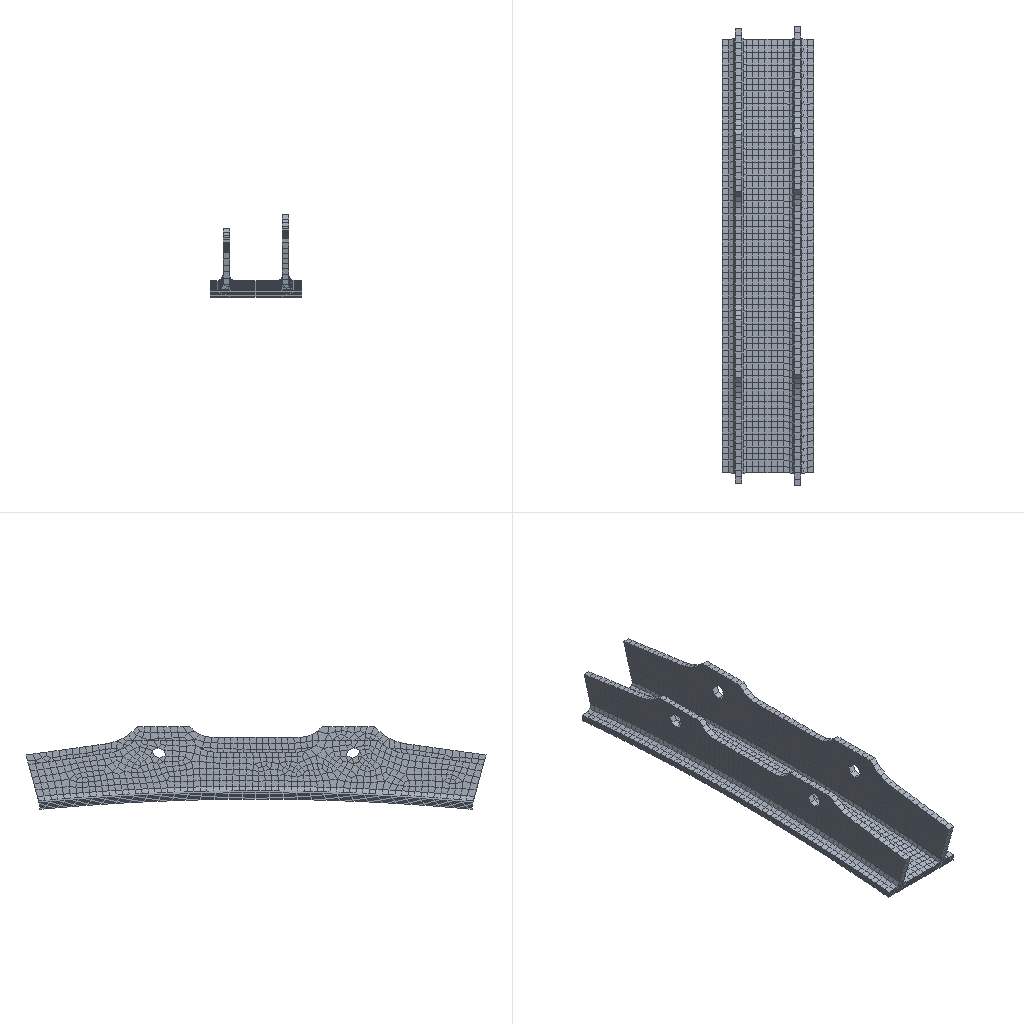Simulation study | abaqus
Set-up summary:
category,name,step,type,value,unit,region
solver,abaqus,,Abaqus/CAE 2024
units,mm-N-s-tonne (MPa),,inferred,E=250000 density=3.2e-09
analysis,Step-1,,coupled temp-displacement,time_period=24
mesh,nodes,,,11334
mesh,elements,,,8250
element_type,C3D8T,,,7245
element_type,COH3D8,,,1005
material,biaoceng,,E,250000
material,biaoceng,,nu,0.17
material,biaoceng,,density,3.2e-09
material,biaoceng,,conductivity,2
material,biaoceng,,specific_heat,7.5e+08
material,biaoceng,,cte,5e-06
material,biaoceng,,behaviors,conductivity; expansion; specific heat
material,bujian,,E,220000
material,bujian,,nu,0.17
material,bujian,,density,1.8e-09
material,bujian,,conductivity,100
material,bujian,,specific_heat,9.6e+08
material,bujian,,cte,4e-06
material,bujian,,behaviors,conductivity; expansion; specific heat
material,cohesive,,E,160000
material,cohesive,,density,2.33e-09
material,cohesive,,conductivity,148
material,cohesive,,specific_heat,7.1e+08
material,cohesive,,cte,4.6e+06
material,cohesive,,behaviors,conductivity; damage initiation; damage evolution; elastic traction; expansion; specific heat
section,bujian,,solid section,,,Set-2
section,biaoceng,,solid section,,,Set-1
section,cohesive,,cohesive section,,,CoheElem-0All
load,Predefined,initial,initial condition temperature
bc,BC-1,Step-1,displacement,1 [dofs=temp],,_PickedSet5
bc,BC-2,Step-1,encastre,[dofs=ENCASTRE],,_PickedSet6
Abaqus input file, long lists of numbers shortened:
*Heading
** Job name: deck Model name: Model-1-Copy
** Generated by: Abaqus/CAE 2024
*Preprint, echo=NO, model=NO, history=NO, contact=NO
**
** PARTS
**
*Part, name=Part1(1)-Surf(Surf-1)
*Node
      1,         -14.,   66.345,  -1.991
      2,          14.,   66.345,  -1.991
** (11332 more lines like these left out)
*Element, type=C3D8T
   1, 12174, 12118, 12182, 11854,     1,    93,  1433,   252
   2, 12118, 12120, 12184, 12182,    93,    94,  1434,  1433
** (7243 more lines like these left out)
*Element, type=COH3D8
7246, 11917, 10901, 10929, 11919, 11918, 10902, 10930, 11920
7247, 10287, 10289, 10317, 10315, 10288, 10290, 10318, 10316
** (1003 more lines like these left out)
*Elset, elset=BaseElements, generate
    1,  7245,     1
*Elset, elset=CoheElem-0All, generate
 7246,  8250,     1
*Elset, elset=Set-1, generate
 1006,  7245,     1
*Elset, elset=Set-2, generate
    1,  1005,     1
** Section: Section-3
*Solid Section, elset=Set-2, material=bujian
,
** Section: Section-1
*Solid Section, elset=Set-1, material=biaoceng
,
** Section: Section-2
*Cohesive Section, elset=CoheElem-0All, material=cohesive, response=TRACTION SEPARATION
,
*End Part
**
**
** ASSEMBLY
**
*Assembly, name=Assembly
**
*Instance, name=Part1(1)-Surf(Surf-1)-1, part=Part1(1)-Surf(Surf-1)
*End Instance
**
*Nset, nset=_PickedSet4, internal, instance=Part1(1)-Surf(Surf-1)-1
     1,     2,     3,     4,     5,     6,     7,     8,     9,    10,    11,    12,    13,    14,    15,    16
    17,    18,    19,    20,    21,    22,    23,    24,    25,    26,    27,    28,    29,    30,    31,    32
** (707 more lines like these left out)
*Nset, nset=_PickedSet5, internal, instance=Part1(1)-Surf(Surf-1)-1
    1,    2,    3,    4,   93,   94,   95,   96,   97,   98,   99,  100,  101,  102,  103,  104
  105,  106,  107,  108,  109,  110,  111,  112,  113,  114,  115,  116,  117,  118,  119,  120
** (66 more lines like these left out)
*Nset, nset=_PickedSet6, internal, instance=Part1(1)-Surf(Surf-1)-1
   33,   34,   37,   38,   46,   47,   50,   51,   65,   66,   69,   70,   77,   78,   81,   82
  774,  775,  776,  777,  778,  779,  780,  781,  800,  801,  802,  803,  804,  805,  806,  807
** (3 more lines like these left out)
*End Assembly
*Amplitude, name=Amp-1
             0.,           1000.,              8.,           1300.,             16.,           1000.,             24.,           1300.
**
** MATERIALS
**
*Material, name=biaoceng
*Conductivity
2.,
*Density
 3.2e-09,
*Elastic
250000., 0.17
*Expansion
 5e-06,
*Specific Heat
 7.5e+08,
*Material, name=bujian
*Conductivity
100.,
*Density
 1.8e-09,
*Elastic
220000., 0.17
*Expansion
 4e-06,
*Specific Heat
 9.6e+08,
*Material, name=cohesive
*Conductivity
148.,
*Damage Initiation, criterion=MAXS
50.,50.,50.
*Damage Evolution, type=DISPLACEMENT
1.,
*Density
 2.33e-09,
*Elastic, type=TRACTION
160000.,160000.,160000.
*Expansion
 4.6e+06,
*Specific Heat
 7.1e+08,
**
** PREDEFINED FIELDS
**
** Name: Predefined Field-1   Type: Temperature
*Initial Conditions, type=TEMPERATURE
_PickedSet4, 1000.
** ----------------------------------------------------------------
**
** STEP: Step-1
**
*Step, name=Step-1, nlgeom=NO, inc=10000
*Coupled Temperature-displacement, creep=none, deltmx=1000., stabilize=0.0002, allsdtol=0.05, continue=NO
0.1, 24., 0.00024, 1.
**
** BOUNDARY CONDITIONS
**
** Name: BC-1 Type: Temperature
*Boundary, amplitude=Amp-1
_PickedSet5, 11, 11, 1.
** Name: BC-2 Type: Symmetry/Antisymmetry/Encastre
*Boundary
_PickedSet6, ENCASTRE
**
** OUTPUT REQUESTS
**
*Restart, write, frequency=0
**
** FIELD OUTPUT: F-Output-1
**
*Output, field
*Node Output
CF, NT, RF, RFL, U
*Element Output, directions=YES
HFL, LE, PE, PEEQ, PEMAG, S, SDEG, STATUS
*Contact Output
CDISP, CSTRESS
**
** HISTORY OUTPUT: H-Output-1
**
*Output, history, variable=PRESELECT
*End Step
Results summary:
result,odb.job_status,,,JOB_STATUS_COMPLETED_SUCCESSFULLY,"consistent, unstated (Abaqus has no unit system)"
result,steps[0].procedure,Step-1,,"*COUPLED TEMPERATURE-DISPLACEMENT, STEADY STATE","consistent, unstated (Abaqus has no unit system)"
result,steps[0].time_period,Step-1,,24,"consistent, unstated (Abaqus has no unit system)"
result,steps[0].n_frames,Step-1,,30,"consistent, unstated (Abaqus has no unit system)"
result,steps[0].last_frame.id,Step-1,,29,"consistent, unstated (Abaqus has no unit system)"
result,steps[0].last_frame.value,Step-1,,24,"consistent, unstated (Abaqus has no unit system)"
result,steps[0].last_frame.description,Step-1,,Increment     29: Step Time =    24.00,"consistent, unstated (Abaqus has no unit system)"
result,steps[0].completed,Step-1,,True,"consistent, unstated (Abaqus has no unit system)"
result,steps[0].max_U_magnitude,Step-1,,0.04372,"consistent, unstated (Abaqus has no unit system)"
result,steps[0].max_S_mises,Step-1,,255.667,"consistent, unstated (Abaqus has no unit system)"
result,steps[0].RF_sum[1],Step-1,,-2.364,"consistent, unstated (Abaqus has no unit system)"
result,steps[0].RF_sum[2],Step-1,,1.16825e-05,"consistent, unstated (Abaqus has no unit system)"
result,steps[0].RF_sum[3],Step-1,,0.07492,"consistent, unstated (Abaqus has no unit system)"